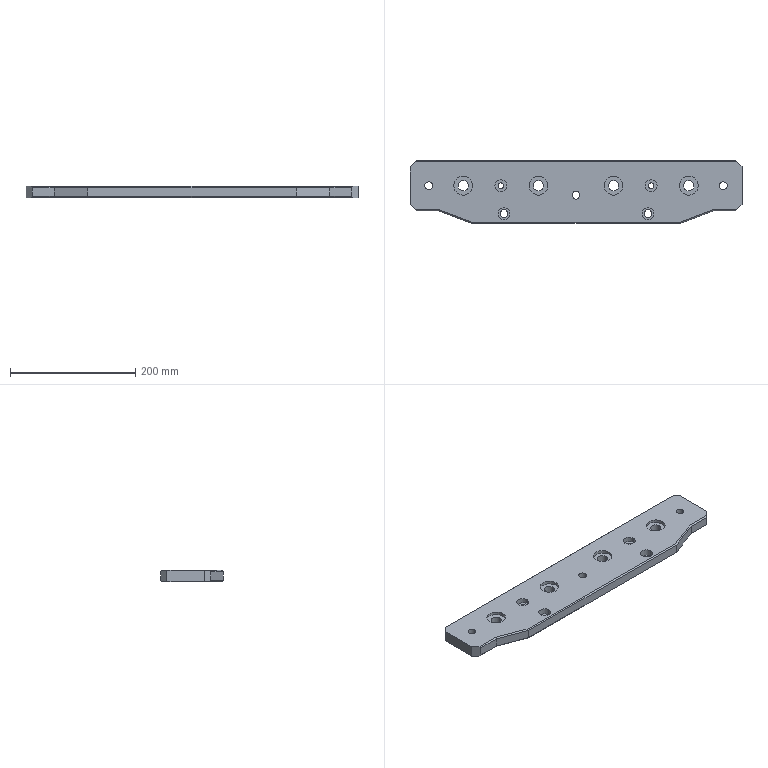Part | SolidWorks | features BaseBody 1 | 1 solid | 78 faces | box 530 x 100 x 18 mm | volume 848525 mm3 | cylinder 42 | plane 36 | commonest cylinder face diameters 12.5 x10 16.5 x8 19 x8 30 x8 9 x4 20.5 x4